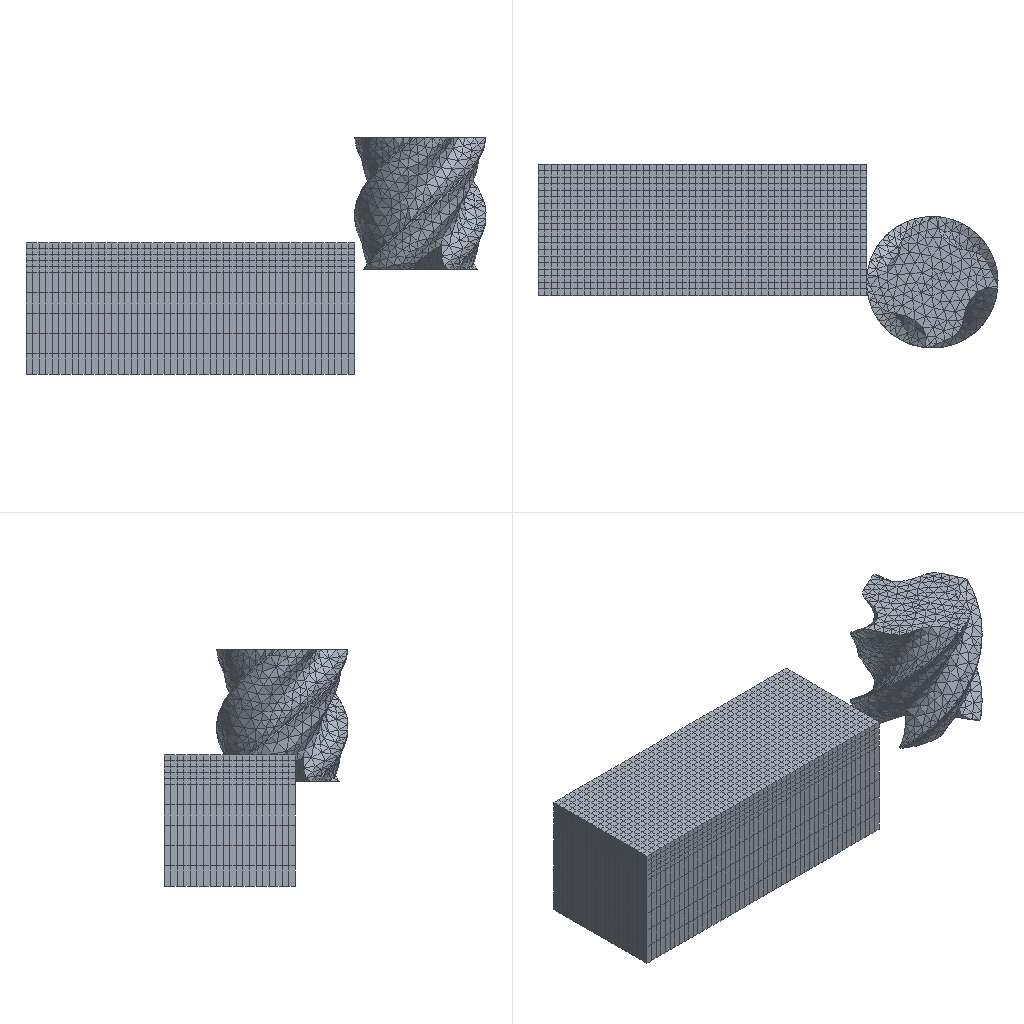Simulation study | abaqus
Set-up summary:
category,name,step,type,value,unit,region
solver,abaqus
solver,version,,,Abaqus/Explicit 2020
units,not stated in the deck,,not stated
analysis,deck,,dynamic temperature-displacement,dynamic temperature-displacement
load_step,Step-1,Step-1,dynamic temperature-displacement,nlgeom=True
contact,interactions,,,general=0 pairs=1 ties=0
load_step,requested,,,1
mesh,nodes,,,13954
mesh,elements,,,19707
element_type,C3D4T,,solid,9707
element_type,C3D8RT,,solid,10000
load,load commands in deck,,count,2
bc,support commands in deck,,count,7
material,MATERIAL-1,,in results
material,TOOL,,in results
check,setup vs results,,match,"per instance, exact: element labels, types and connectivity; labels of the nodes the elements use; coordinates of those nodes at SINGLE_PRECISION in 1 of 2 instance(s)"
Abaqus input file, long lists of numbers shortened:
*Heading
** Job name: Job-1 Model name: Model-1
** Generated by: Abaqus/CAE 2020
*Preprint, echo=NO, model=NO, history=NO, contact=NO
**
** PARTS
**
*Part, name=tool
*Node
      1,   17.835,  -22.287,   16.894
      2,         14.5,        -20.5,          16.
** (2171 more lines like these left out)
*Element, type=C3D4T
   1, 1033, 1034, 1035, 1036
   2, 1033, 1037, 1038, 1039
** (9705 more lines like these left out)
*Nset, nset=Set-5, generate
    1,  2173,     1
*Elset, elset=Set-5, generate
    1,  9707,     1
** Section: tool
*Solid Section, elset=Set-5, material=tool
,
*End Part
**
*Part, name=work
*Node
      1,         -50.,         -20.,         15.5
      2,         -50.,           0.,         15.5
** (11779 more lines like these left out)
*Element, type=C3D8RT
   1,  202,  997, 4334,  605,    1,   13,  453,   58
   2,  997,  998, 4335, 4334,   13,   14,  454,  453
** (9998 more lines like these left out)
*Nset, nset=Set-4, generate
     1,  11781,      1
*Elset, elset=Set-4, generate
     1,  10000,      1
** Section: Section-1
*Solid Section, elset=Set-4, material=Material-1
,
*End Part
**
**
** ASSEMBLY
**
*Assembly, name=Assembly
**
*Instance, name=zhuangpei-1-1, part=work
        -10.,          18.,         -36.
*End Instance
**
*Instance, name=zhuangpei-2-1, part=tool
-19.392, 9.588,         -36.
-19.392, 9.588,         -36., -19.392, 9.588, -35., 30.
*End Instance
**
*Node
      1,           0.,           0.,           0.
*Nset, nset=Set-2, instance=zhuangpei-1-1
    1,    2,    3,    4,    6,    7,   13,   14,   15,   16,   17,   18,   19,   20,   21,   22
   23,   24,   25,   26,   27,   28,   29,   30,   31,   32,   33,   34,   35,   36,   37,   38
** (72 more lines like these left out)
*Elset, elset=Set-2, instance=zhuangpei-1-1
    1,    2,    3,    4,    5,    6,    7,    8,    9,   10,   11,   12,   13,   14,   15,   16
   17,   18,   19,   20,   21,   22,   23,   24,   25,   26,   27,   28,   29,   30,   31,   32
** (66 more lines like these left out)
*Nset, nset=Set-3
 1,
*Nset, nset=b_Set-4, instance=zhuangpei-2-1, generate
    1,  2173,     1
*Elset, elset=b_Set-4, instance=zhuangpei-2-1, generate
    1,  9707,     1
*Nset, nset=s_Set-1, instance=zhuangpei-1-1
     1,     2,     5,     8,     9,    10,    11,    12,    13,    14,    15,    16,    17,    18,    19,    20
    21,    22,    23,    24,    25,    26,    27,    28,    29,    30,    31,    59,    60,    61,    62,    63
** (400 more lines like these left out)
*Elset, elset=s_Set-1, instance=zhuangpei-1-1
     1,     2,     3,     4,     5,     6,     7,     8,     9,    10,    11,    12,    13,    14,    15,    16
    17,    18,    19,    20,   101,   102,   103,   104,   105,   106,   107,   108,   109,   110,   111,   112
** (373 more lines like these left out)
*Nset, nset=_PickedSet12, internal
 1,
*Elset, elset=_m_Surf-1_S3, internal, instance=zhuangpei-2-1
   77,   83,  113,  137,  225,  312,  360,  400,  464,  466,  544,  546,  562,  582,  586,  594
  625,  666,  676,  733,  875,  888,  894,  924,  956, 1047, 1138, 1179, 1188, 1208, 1248, 1376
** (94 more lines like these left out)
*Elset, elset=_m_Surf-1_S1, internal, instance=zhuangpei-2-1
  335,  734,  956, 1563, 1639, 1704, 1743, 1816, 2037, 2073, 2076, 2083, 2110, 2180, 2215, 2296
 2361, 2365, 2378, 2395, 2425, 2446, 2465, 2510, 2612, 2675, 2750, 2837, 2865, 2882, 3100, 3161
** (8 more lines like these left out)
*Elset, elset=_m_Surf-1_S4, internal, instance=zhuangpei-2-1
    4,   46,  676,  927, 1509, 1639, 1688, 1764, 1861, 1900, 1922, 1933, 1984, 2025, 2043, 2052
 2104, 2142, 2233, 2299, 2338, 2370, 2374, 2379, 2497, 2561, 2581, 2669, 2670, 2716, 2764, 2765
** (9 more lines like these left out)
*Elset, elset=_m_Surf-1_S2, internal, instance=zhuangpei-2-1
   20,   52,  130,  171,  214,  312,  544,  546,  677,  734, 1467, 1651, 1652, 1720, 1798, 1814
 1815, 1872, 1923, 1933, 1954, 1969, 1997, 2055, 2080, 2115, 2179, 2229, 2260, 2319, 2332, 2338
** (12 more lines like these left out)
*Surface, type=ELEMENT, name=m_Surf-1
_m_Surf-1_S3, S3
_m_Surf-1_S1, S1
_m_Surf-1_S4, S4
_m_Surf-1_S2, S2
*Surface, type=NODE, name=s_Set-1_CNS_, internal
s_Set-1, 1.
** Constraint: Constraint-1
*Rigid Body, ref node=_PickedSet12, elset=b_Set-4
*End Assembly
**
** MATERIALS
**
*Material, name=Material-1
*Conductivity
44.,
*Damage Initiation, criterion=SHEAR
 0.5,0.,0.
*Damage Evolution, type=DISPLACEMENT
 0.01,
*Density
 7.85e-09,
*Elastic
200000., 0.33
*Plastic
121.,0.
*Specific Heat
 4.6e+08,
*Material, name=tool
*Conductivity
46.,
*Density
 1.5e-08,
*Elastic
800000., 0.23
*Expansion
 4.7e-06,
*Specific Heat
 2.03e+08,
**
** INTERACTION PROPERTIES
**
*Surface Interaction, name=IntProp-1
*Friction
 0.15,
*Surface Behavior, pressure-overclosure=HARD
*Gap Conductance
1000.,  0.
   0., 0.1
** ----------------------------------------------------------------
**
** STEP: Step-1
**
*Step, name=Step-1, nlgeom=YES
*Dynamic Temperature-displacement, Explicit
, 0.1
*Bulk Viscosity
0.06, 1.2
** Mass Scaling: Semi-Automatic
**               Whole Model
*Fixed Mass Scaling, factor=500.
**
** BOUNDARY CONDITIONS
**
** Name: BC-1 Type: 对称/反对称/完全固定
*Boundary
Set-2, ENCASTRE
** Name: [REDACTED] : Velocity/Angular velocity
*Boundary, type=VELOCITY
Set-3, 1, 1, -600.
Set-3, 2, 2
Set-3, 3, 3
Set-3, 4, 4
Set-3, 5, 5
Set-3, 6, 6, -200.
**
** INTERACTIONS
**
** Interaction: Int-1
*Contact Pair, interaction=IntProp-1, mechanical constraint=KINEMATIC, cpset=Int-1
m_Surf-1, s_Set-1_CNS_
**
** OUTPUT REQUESTS
**
*Restart, write, number interval=1, time marks=NO
**
** FIELD OUTPUT: F-Output-1
**
*Output, field, number interval=30
*Node Output
A, CF, NT, RF, RFL, RM, RT, U
V
*Element Output, directions=YES
E, EVF, HFL, LE, MISES, MISESMAX, MISESONLY, PE, PEEQ, PEEQMAX, PEEQT, PEEQVAVG, PEMAG, PEVAVG, PRESSONLY, S
SEQUT, SF, SSAVG, STATUS, SVAVG, TEMP, TSHR, YIELDPOT
*Contact Output
CDISP, CSTRESS, HFLA, HTL
**
** HISTORY OUTPUT: H-Output-1
**
*Output, history, time interval=2e-06
*Node Output, nset=Set-3
RF1, RF2, RF3, RM1, RM2, RM3
*End Step
Results summary:
result,step,Step-1,completed,increments=42308 time=0.1/0.1
result,analysis,,,"dynamic temperature-displacement, explict"
result,last_loadstep,,,1
result,analysis steps,,count,1
result,primary field,,,"U, NT11"
result,reaction total,,FX,811.559,model units
result,reaction total,,FY,1060.601,model units
result,reaction total,,FZ,1293.873,model units